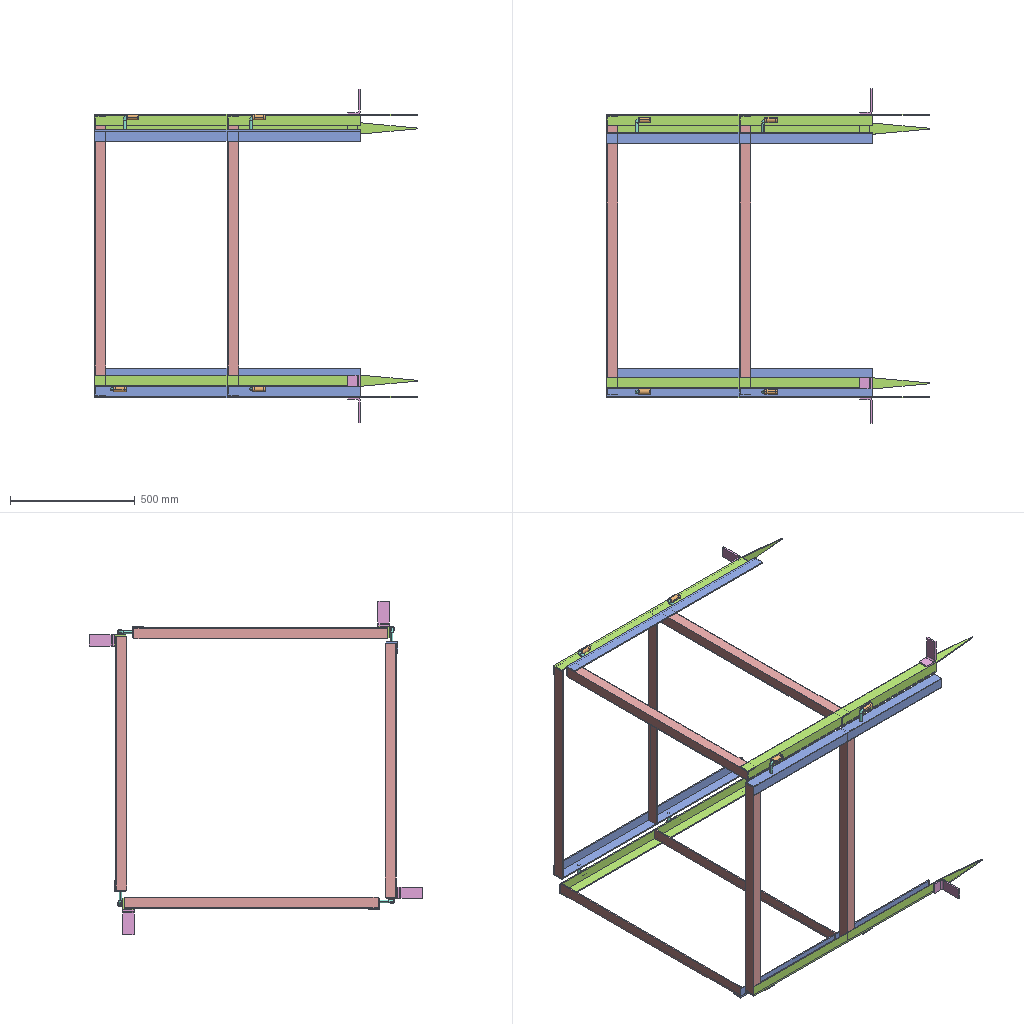Assembly | SolidWorks | 6 different items | 36 placed | box 1295 x 1339 x 1339 mm
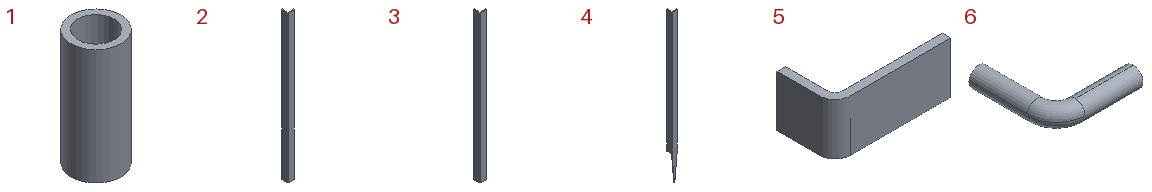Parts list (item | quantity | size | volume | features):
1 | x8 | 22 x 22 x 50.8 mm | 9097 mm3 | features Extrusion 1
2 | x8 | 45 x 45 x 1019 mm | 432947 mm3 | features Extrusion 1
3 | x4 | 45 x 45 x 1067 mm | 453390 mm3 | features Extrusion 1
4 | x4 | 45 x 45 x 1295 mm | 480925 mm3 | features ICE 2, Extrusion 1
5 | x4 | 101.6 x 50.8 x 45 mm | 47441 mm3 | features Extrusion 1
6 | x8 | 57.15 x 57.15 x 12.7 mm | 12180 mm3 | features 3DProfileFeature 1, Sweep 1
Mates (type | each side: item.copy, entity, surface, feature):
Coincident | 2.1 face plane Extrude1 | 3.1 face plane Extrude1 | 3 times
Coincident | 4.1 face plane Extrude1 | 2.2 face plane Extrude1 | 2 times
DistanceDim | 2.2 face plane Extrude1 | 2.1 face plane Extrude1
Coincident | 4.1 face plane Extrude1 | 5.1 face plane Extrude1
Coincident | 5.1 face plane Extrude1 | 4.1 face plane Extrude1
Coincident | 4.1 face plane Extrude3 | 5.1 face plane Extrude1
DistanceDim | 3.1 face plane Extrude1 | 6.1 face plane Sweep8
Coincident | 2.1 face plane Extrude1 | 4.1 face plane Extrude1 | 3 times
DistanceDim | 6.1 select_type:0 | 2.1 face plane Extrude1
DistanceDim | 6.1 plane | 3.1 face plane Extrude1
Coincident | 3.1 face plane Extrude1 | 6.2 face plane Sweep8
DistanceDim | 6.2 select_type:0 | 2.1 face plane Extrude1
DistanceDim | 6.2 plane | 3.1 face plane Extrude1
DistanceDim | 1.1 face plane Extrude1 | 2.1 face plane Extrude1
DistanceDim | 1.1 plane | 4.1 face plane Extrude1 | 2 times
DistanceDim | 1.2 face plane Extrude1 | 2.1 face plane Extrude1
Tangent | 4.1 face plane Extrude1 | 1.2 face cylinder Extrude1
DistanceDim | 1.2 plane | 4.1 face plane Extrude1
Parallel | 6.1 select_type:0 | 1.3 face plane Extrude1
Concentric | 6.1 face cylinder Sweep8 | 1.3 face cylinder Extrude1
Tangent | 6.1 face torus Sweep8 | 1.3 face plane Extrude1
Parallel | 6.2 face plane Sweep8 | 1.4 face plane Extrude1
Concentric | 6.2 face cylinder Sweep8 | 1.4 face cylinder Extrude1
Tangent | 6.2 face torus Sweep8 | 1.4 face plane Extrude1
Tangent | 1.3 face cylinder Extrude1 | 4.2 face plane Extrude1
DistanceDim | 1.3 face plane Extrude1 | 4.2 face plane Extrude1
DistanceDim | 4.2 face plane Extrude1 | 1.3 plane
Parallel | 3.1 face plane Extrude1 | 4.2 face plane Extrude1
Coincident | 4.2 face plane Extrude1 | 2.3 face plane Extrude1 | 3 times
Coincident | 4.2 face plane Extrude1 | 2.4 face plane Extrude1 | 2 times
DistanceDim | 2.4 face plane Extrude1 | 2.3 face plane Extrude1
Coincident | 2.3 face plane Extrude1 | 3.2 face plane Extrude1 | 3 times
Coincident | 4.2 face plane Extrude1 | 5.2 face plane Extrude1 | 2 times
Coincident | 4.2 face plane Extrude3 | 5.2 face plane Extrude1
Coincident | 3.2 face plane Extrude1 | 6.3 face plane Sweep8
DistanceDim | 2.3 face plane Extrude1 | 6.3 select_type:0
DistanceDim | 3.2 face plane Extrude1 | 6.3 plane
Coincident | 6.4 face plane Sweep8 | 3.2 face plane Extrude1
DistanceDim | 6.4 face plane Sweep8 | 2.3 face plane Extrude1
DistanceDim | 3.2 face plane Extrude1 | 6.4 plane
Parallel | 2.3 face plane Extrude1 | 1.5 face plane Extrude1
Concentric | 6.3 face cylinder Sweep8 | 1.5 face cylinder Extrude1
Tangent | 6.3 face torus Sweep8 | 1.5 face plane Extrude1
Concentric | 6.4 face cylinder Sweep8 | 1.6 face cylinder Extrude1
Tangent | 6.4 face torus Sweep8 | 1.6 face plane Extrude1
Tangent | 1.5 face cylinder Extrude1 | 4.3 face plane Extrude1 | 2 times
DistanceDim | 4.3 face plane Extrude1 | 1.5 face plane Extrude1
Parallel | 6.3 plane | 4.3 face plane Extrude1
DistanceDim | 1.5 plane | 4.3 face plane Extrude1
Coincident | 4.3 face plane Extrude1 | 2.5 face plane Extrude1 | 3 times
Coincident | 4.3 face plane Extrude1 | 2.6 face plane Extrude1 | 2 times
DistanceDim | 2.6 face plane Extrude1 | 2.5 face plane Extrude1
Coincident | 2.5 face plane Extrude1 | 3.3 face plane Extrude1 | 3 times
Coincident | 4.3 face plane Extrude1 | 5.3 face plane Extrude1 | 2 times
Coincident | 4.3 face plane Extrude3 | 5.3 face plane Extrude1
Coincident | 3.3 face plane Extrude1 | 6.5 face plane Sweep8
DistanceDim | 2.5 face plane Extrude1 | 6.5 select_type:0
DistanceDim | 6.5 plane | 3.3 face plane Extrude1
Coincident | 3.3 face plane Extrude1 | 6.6 face plane Sweep8
DistanceDim | 2.5 face plane Extrude1 | 6.6 select_type:0
DistanceDim | 3.3 face plane Extrude1 | 6.6 plane
Concentric | 6.5 face cylinder Sweep8 | 1.7 face cylinder Extrude1
Tangent | 6.5 face torus Sweep8 | 1.7 face plane Extrude1
Concentric | 6.6 face cylinder Sweep8 | 1.8 face cylinder Extrude1
Tangent | 1.8 face plane Extrude1 | 6.6 face torus Sweep8
Tangent | 1.7 face cylinder Extrude1 | 4.4 face plane Extrude1
Parallel | 3.3 face plane Extrude1 | 4.4 face plane Extrude1
Coincident | 2.5 face plane Extrude1 | 4.4 face plane Extrude1
DistanceDim | 4.4 face plane Extrude1 | 1.7 plane
Coincident | 4.4 face plane Extrude1 | 2.7 face plane Extrude1 | 3 times
Coincident | 4.4 face plane Extrude1 | 2.8 face plane Extrude1 | 2 times
DistanceDim | 2.7 face plane Extrude1 | 2.8 face plane Extrude1
Coincident | 2.7 face plane Extrude1 | 3.4 face plane Extrude1 | 3 times
Concentric | 1.1 face cylinder Extrude1 | 6.7 face cylinder Sweep8
Tangent | 6.7 face torus Sweep8 | 1.1 face plane Extrude1
Parallel | 6.7 face plane Sweep8 | 3.4 face plane Extrude1
Concentric | 1.2 face cylinder Extrude1 | 6.8 face cylinder Sweep8
Tangent | 1.2 face plane Extrude1 | 6.8 face torus Sweep8
Parallel | 3.4 face plane Extrude1 | 6.8 face plane Sweep8
Coincident | 4.4 face plane Extrude1 | 5.4 face plane Extrude1
Coincident | 5.4 face plane Extrude1 | 4.4 face plane Extrude1
Coincident | 4.4 face plane Extrude3 | 5.4 face plane Extrude1